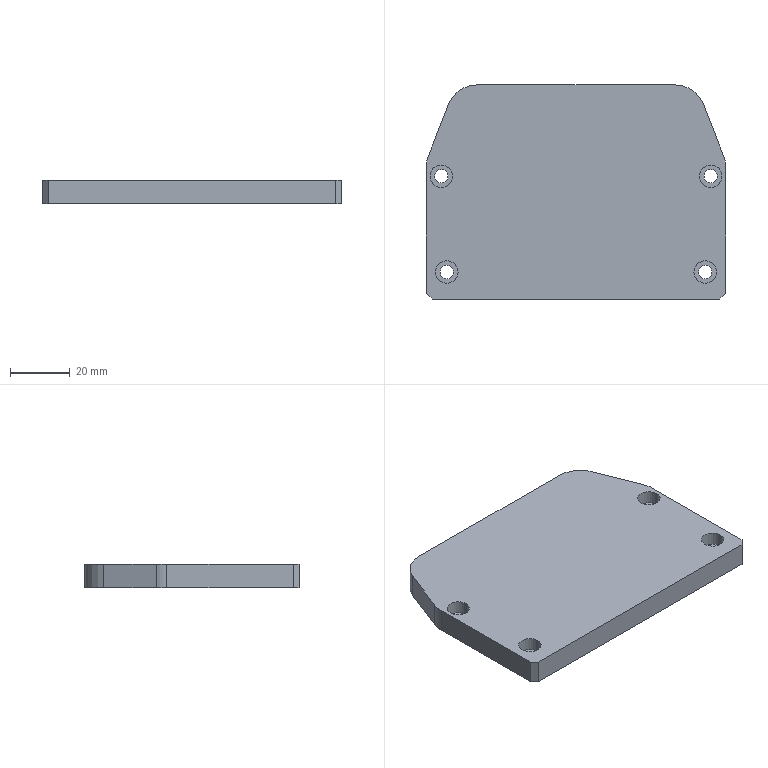Part | SolidWorks | features Chamfer 1, Cut 1, Extrusion 1, Fillet 1, HoleWzd 1, ICE 1 | 1 solid | 37 faces | box 100 x 71.5 x 8 mm | volume 49163 mm3 | cylinder 22 | plane 15 | commonest cylinder face diameters 4.5 x8 7.5 x8 20 x4 35 x2
STEP:
#1=CARTESIAN_POINT('',(-48.75,5.25,3.5));
#2=VERTEX_POINT('',#1);
#3=CARTESIAN_POINT('',(-41.25,5.25,3.5));
#4=VERTEX_POINT('',#3);
#5=CARTESIAN_POINT('',(-45.,5.25,3.5));
#6=DIRECTION('',(0.,0.,1.));
#7=DIRECTION('',(1.,0.,0.));
#8=AXIS2_PLACEMENT_3D('',#5,#6,#7);
#9=CIRCLE('',#8,3.75);
#10=EDGE_CURVE('',#2,#4,#9,.T.);
#11=ORIENTED_EDGE('',*,*,#10,.F.);
#12=CARTESIAN_POINT('',(-48.75,5.25,8.));
#13=VERTEX_POINT('',#12);
#14=CARTESIAN_POINT('',(-48.75,5.25,8.));
#15=DIRECTION('',(0.,0.,1.));
#16=VECTOR('',#15,1000.);
#17=LINE('',#14,#16);
#18=EDGE_CURVE('',#2,#13,#17,.T.);
#19=ORIENTED_EDGE('',*,*,#18,.T.);
#20=CARTESIAN_POINT('',(-41.25,5.25,8.));
#21=VERTEX_POINT('',#20);
#22=CARTESIAN_POINT('',(-45.,5.25,8.));
#23=DIRECTION('',(0.,0.,1.));
#24=DIRECTION('',(1.,0.,0.));
#25=AXIS2_PLACEMENT_3D('',#22,#23,#24);
#26=CIRCLE('',#25,3.75);
#27=EDGE_CURVE('',#13,#21,#26,.T.);
#28=ORIENTED_EDGE('',*,*,#27,.T.);
#29=CARTESIAN_POINT('',(-41.25,5.25,8.));
#30=DIRECTION('',(0.,0.,1.));
#31=VECTOR('',#30,1000.);
#32=LINE('',#29,#31);
#33=EDGE_CURVE('',#4,#21,#32,.T.);
#34=ORIENTED_EDGE('',*,*,#33,.F.);
#35=EDGE_LOOP('',(#11,#19,#28,#34));
#36=FACE_OUTER_BOUND('',#35,.T.);
#37=CARTESIAN_POINT('',(-45.,5.25,8.));
#38=DIRECTION('',(0.,0.,1.));
#39=DIRECTION('',(1.,0.,0.));
#40=AXIS2_PLACEMENT_3D('',#37,#38,#39);
#41=CYLINDRICAL_SURFACE('',#40,3.75);
#42=ADVANCED_FACE('',(#36),#41,.F.);
#43=CARTESIAN_POINT('',(-47.25,5.25,0.));
#44=VERTEX_POINT('',#43);
#45=CARTESIAN_POINT('',(-42.75,5.25,0.));
#46=VERTEX_POINT('',#45);
#47=CARTESIAN_POINT('',(-45.,5.25,0.));
#48=DIRECTION('',(0.,0.,1.));
#49=DIRECTION('',(1.,0.,0.));
#50=AXIS2_PLACEMENT_3D('',#47,#48,#49);
#51=CIRCLE('',#50,2.25);
#52=EDGE_CURVE('',#44,#46,#51,.T.);
#53=ORIENTED_EDGE('',*,*,#52,.F.);
#54=CARTESIAN_POINT('',(-47.25,5.25,3.5));
#55=VERTEX_POINT('',#54);
#56=CARTESIAN_POINT('',(-47.25,5.25,8.));
#57=DIRECTION('',(0.,0.,1.));
#58=VECTOR('',#57,1000.);
#59=LINE('',#56,#58);
#60=EDGE_CURVE('',#44,#55,#59,.T.);
#61=ORIENTED_EDGE('',*,*,#60,.T.);
#62=CARTESIAN_POINT('',(-42.75,5.25,3.5));
#63=VERTEX_POINT('',#62);
#64=CARTESIAN_POINT('',(-45.,5.25,3.5));
#65=DIRECTION('',(0.,0.,1.));
#66=DIRECTION('',(1.,0.,0.));
#67=AXIS2_PLACEMENT_3D('',#64,#65,#66);
#68=CIRCLE('',#67,2.25);
#69=EDGE_CURVE('',#55,#63,#68,.T.);
#70=ORIENTED_EDGE('',*,*,#69,.T.);
#71=CARTESIAN_POINT('',(-42.75,5.25,8.));
#72=DIRECTION('',(0.,0.,1.));
#73=VECTOR('',#72,1000.);
#74=LINE('',#71,#73);
#75=EDGE_CURVE('',#46,#63,#74,.T.);
#76=ORIENTED_EDGE('',*,*,#75,.F.);
#77=EDGE_LOOP('',(#53,#61,#70,#76));
#78=FACE_OUTER_BOUND('',#77,.T.);
#79=CARTESIAN_POINT('',(-45.,5.25,8.));
#80=DIRECTION('',(0.,0.,1.));
#81=DIRECTION('',(1.,0.,0.));
#82=AXIS2_PLACEMENT_3D('',#79,#80,#81);
#83=CYLINDRICAL_SURFACE('',#82,2.25);
#84=ADVANCED_FACE('',(#78),#83,.F.);
#85=CARTESIAN_POINT('',(-46.9,-26.75,3.5));
#86=VERTEX_POINT('',#85);
#87=CARTESIAN_POINT('',(-39.4,-26.75,3.5));
#88=VERTEX_POINT('',#87);
#89=CARTESIAN_POINT('',(-43.15,-26.75,3.5));
#90=DIRECTION('',(0.,0.,1.));
#91=DIRECTION('',(1.,0.,0.));
#92=AXIS2_PLACEMENT_3D('',#89,#90,#91);
#93=CIRCLE('',#92,3.75);
#94=EDGE_CURVE('',#86,#88,#93,.T.);
#95=ORIENTED_EDGE('',*,*,#94,.F.);
#96=CARTESIAN_POINT('',(-46.9,-26.75,8.));
#97=VERTEX_POINT('',#96);
#98=CARTESIAN_POINT('',(-46.9,-26.75,8.));
#99=DIRECTION('',(0.,0.,1.));
#100=VECTOR('',#99,1000.);
#101=LINE('',#98,#100);
#102=EDGE_CURVE('',#86,#97,#101,.T.);
#103=ORIENTED_EDGE('',*,*,#102,.T.);
#104=CARTESIAN_POINT('',(-39.4,-26.75,8.));
#105=VERTEX_POINT('',#104);
#106=CARTESIAN_POINT('',(-43.15,-26.75,8.));
#107=DIRECTION('',(0.,0.,1.));
#108=DIRECTION('',(1.,0.,0.));
#109=AXIS2_PLACEMENT_3D('',#106,#107,#108);
#110=CIRCLE('',#109,3.75);
#111=EDGE_CURVE('',#97,#105,#110,.T.);
#112=ORIENTED_EDGE('',*,*,#111,.T.);
#113=CARTESIAN_POINT('',(-39.4,-26.75,8.));
#114=DIRECTION('',(0.,0.,1.));
#115=VECTOR('',#114,1000.);
#116=LINE('',#113,#115);
#117=EDGE_CURVE('',#88,#105,#116,.T.);
#118=ORIENTED_EDGE('',*,*,#117,.F.);
#119=EDGE_LOOP('',(#95,#103,#112,#118));
#120=FACE_OUTER_BOUND('',#119,.T.);
#121=CARTESIAN_POINT('',(-43.15,-26.75,8.));
#122=DIRECTION('',(0.,0.,1.));
#123=DIRECTION('',(1.,0.,0.));
#124=AXIS2_PLACEMENT_3D('',#121,#122,#123);
#125=CYLINDRICAL_SURFACE('',#124,3.75);
#126=ADVANCED_FACE('',(#120),#125,.F.);
#127=CARTESIAN_POINT('',(-45.4,-26.75,0.));
#128=VERTEX_POINT('',#127);
#129=CARTESIAN_POINT('',(-40.9,-26.75,0.));
#130=VERTEX_POINT('',#129);
#131=CARTESIAN_POINT('',(-43.15,-26.75,0.));
#132=DIRECTION('',(0.,0.,1.));
#133=DIRECTION('',(1.,0.,0.));
#134=AXIS2_PLACEMENT_3D('',#131,#132,#133);
#135=CIRCLE('',#134,2.25);
#136=EDGE_CURVE('',#128,#130,#135,.T.);
#137=ORIENTED_EDGE('',*,*,#136,.F.);
#138=CARTESIAN_POINT('',(-45.4,-26.75,3.5));
#139=VERTEX_POINT('',#138);
#140=CARTESIAN_POINT('',(-45.4,-26.75,8.));
#141=DIRECTION('',(0.,0.,1.));
#142=VECTOR('',#141,1000.);
#143=LINE('',#140,#142);
#144=EDGE_CURVE('',#128,#139,#143,.T.);
#145=ORIENTED_EDGE('',*,*,#144,.T.);
#146=CARTESIAN_POINT('',(-40.9,-26.75,3.5));
#147=VERTEX_POINT('',#146);
#148=CARTESIAN_POINT('',(-43.15,-26.75,3.5));
#149=DIRECTION('',(0.,0.,1.));
#150=DIRECTION('',(1.,0.,0.));
#151=AXIS2_PLACEMENT_3D('',#148,#149,#150);
#152=CIRCLE('',#151,2.25);
#153=EDGE_CURVE('',#139,#147,#152,.T.);
#154=ORIENTED_EDGE('',*,*,#153,.T.);
#155=CARTESIAN_POINT('',(-40.9,-26.75,8.));
#156=DIRECTION('',(0.,0.,1.));
#157=VECTOR('',#156,1000.);
#158=LINE('',#155,#157);
#159=EDGE_CURVE('',#130,#147,#158,.T.);
#160=ORIENTED_EDGE('',*,*,#159,.F.);
#161=EDGE_LOOP('',(#137,#145,#154,#160));
#162=FACE_OUTER_BOUND('',#161,.T.);
#163=CARTESIAN_POINT('',(-43.15,-26.75,8.));
#164=DIRECTION('',(0.,0.,1.));
#165=DIRECTION('',(1.,0.,0.));
#166=AXIS2_PLACEMENT_3D('',#163,#164,#165);
#167=CYLINDRICAL_SURFACE('',#166,2.25);
#168=ADVANCED_FACE('',(#162),#167,.F.);
#169=CARTESIAN_POINT('',(41.25,5.25,3.5));
#170=VERTEX_POINT('',#169);
#171=CARTESIAN_POINT('',(48.75,5.25,3.5));
#172=VERTEX_POINT('',#171);
#173=CARTESIAN_POINT('',(45.,5.25,3.5));
#174=DIRECTION('',(0.,0.,1.));
#175=DIRECTION('',(1.,0.,0.));
#176=AXIS2_PLACEMENT_3D('',#173,#174,#175);
#177=CIRCLE('',#176,3.75);
#178=EDGE_CURVE('',#170,#172,#177,.T.);
#179=ORIENTED_EDGE('',*,*,#178,.F.);
#180=CARTESIAN_POINT('',(41.25,5.25,8.));
#181=VERTEX_POINT('',#180);
#182=CARTESIAN_POINT('',(41.25,5.25,8.));
#183=DIRECTION('',(0.,0.,1.));
#184=VECTOR('',#183,1000.);
#185=LINE('',#182,#184);
#186=EDGE_CURVE('',#170,#181,#185,.T.);
#187=ORIENTED_EDGE('',*,*,#186,.T.);
#188=CARTESIAN_POINT('',(48.75,5.25,8.));
#189=VERTEX_POINT('',#188);
#190=CARTESIAN_POINT('',(45.,5.25,8.));
#191=DIRECTION('',(0.,0.,1.));
#192=DIRECTION('',(1.,0.,0.));
#193=AXIS2_PLACEMENT_3D('',#190,#191,#192);
#194=CIRCLE('',#193,3.75);
#195=EDGE_CURVE('',#181,#189,#194,.T.);
#196=ORIENTED_EDGE('',*,*,#195,.T.);
#197=CARTESIAN_POINT('',(48.75,5.25,8.));
#198=DIRECTION('',(0.,0.,1.));
#199=VECTOR('',#198,1000.);
#200=LINE('',#197,#199);
#201=EDGE_CURVE('',#172,#189,#200,.T.);
#202=ORIENTED_EDGE('',*,*,#201,.F.);
#203=EDGE_LOOP('',(#179,#187,#196,#202));
#204=FACE_OUTER_BOUND('',#203,.T.);
#205=CARTESIAN_POINT('',(45.,5.25,8.));
#206=DIRECTION('',(0.,0.,1.));
#207=DIRECTION('',(1.,0.,0.));
#208=AXIS2_PLACEMENT_3D('',#205,#206,#207);
#209=CYLINDRICAL_SURFACE('',#208,3.75);
#210=ADVANCED_FACE('',(#204),#209,.F.);
#211=CARTESIAN_POINT('',(42.75,5.25,0.));
#212=VERTEX_POINT('',#211);
#213=CARTESIAN_POINT('',(47.25,5.25,0.));
#214=VERTEX_POINT('',#213);
#215=CARTESIAN_POINT('',(45.,5.25,0.));
#216=DIRECTION('',(0.,0.,1.));
#217=DIRECTION('',(1.,0.,0.));
#218=AXIS2_PLACEMENT_3D('',#215,#216,#217);
#219=CIRCLE('',#218,2.25);
#220=EDGE_CURVE('',#212,#214,#219,.T.);
#221=ORIENTED_EDGE('',*,*,#220,.F.);
#222=CARTESIAN_POINT('',(42.75,5.25,3.5));
#223=VERTEX_POINT('',#222);
#224=CARTESIAN_POINT('',(42.75,5.25,8.));
#225=DIRECTION('',(0.,0.,1.));
#226=VECTOR('',#225,1000.);
#227=LINE('',#224,#226);
#228=EDGE_CURVE('',#212,#223,#227,.T.);
#229=ORIENTED_EDGE('',*,*,#228,.T.);
#230=CARTESIAN_POINT('',(47.25,5.25,3.5));
#231=VERTEX_POINT('',#230);
#232=CARTESIAN_POINT('',(45.,5.25,3.5));
#233=DIRECTION('',(0.,0.,1.));
#234=DIRECTION('',(1.,0.,0.));
#235=AXIS2_PLACEMENT_3D('',#232,#233,#234);
#236=CIRCLE('',#235,2.25);
#237=EDGE_CURVE('',#223,#231,#236,.T.);
#238=ORIENTED_EDGE('',*,*,#237,.T.);
#239=CARTESIAN_POINT('',(47.25,5.25,8.));
#240=DIRECTION('',(0.,0.,1.));
#241=VECTOR('',#240,1000.);
#242=LINE('',#239,#241);
#243=EDGE_CURVE('',#214,#231,#242,.T.);
#244=ORIENTED_EDGE('',*,*,#243,.F.);
#245=EDGE_LOOP('',(#221,#229,#238,#244));
#246=FACE_OUTER_BOUND('',#245,.T.);
#247=CARTESIAN_POINT('',(45.,5.25,8.));
#248=DIRECTION('',(0.,0.,1.));
#249=DIRECTION('',(1.,0.,0.));
#250=AXIS2_PLACEMENT_3D('',#247,#248,#249);
#251=CYLINDRICAL_SURFACE('',#250,2.25);
#252=ADVANCED_FACE('',(#246),#251,.F.);
#253=CARTESIAN_POINT('',(39.4,-26.75,3.5));
#254=VERTEX_POINT('',#253);
#255=CARTESIAN_POINT('',(46.9,-26.75,3.5));
#256=VERTEX_POINT('',#255);
#257=CARTESIAN_POINT('',(43.15,-26.75,3.5));
#258=DIRECTION('',(0.,0.,1.));
#259=DIRECTION('',(1.,0.,0.));
#260=AXIS2_PLACEMENT_3D('',#257,#258,#259);
#261=CIRCLE('',#260,3.75);
#262=EDGE_CURVE('',#254,#256,#261,.T.);
#263=ORIENTED_EDGE('',*,*,#262,.F.);
#264=CARTESIAN_POINT('',(39.4,-26.75,8.));
#265=VERTEX_POINT('',#264);
#266=CARTESIAN_POINT('',(39.4,-26.75,8.));
#267=DIRECTION('',(0.,0.,1.));
#268=VECTOR('',#267,1000.);
#269=LINE('',#266,#268);
#270=EDGE_CURVE('',#254,#265,#269,.T.);
#271=ORIENTED_EDGE('',*,*,#270,.T.);
#272=CARTESIAN_POINT('',(46.9,-26.75,8.));
#273=VERTEX_POINT('',#272);
#274=CARTESIAN_POINT('',(43.15,-26.75,8.));
#275=DIRECTION('',(0.,0.,1.));
#276=DIRECTION('',(1.,0.,0.));
#277=AXIS2_PLACEMENT_3D('',#274,#275,#276);
#278=CIRCLE('',#277,3.75);
#279=EDGE_CURVE('',#265,#273,#278,.T.);
#280=ORIENTED_EDGE('',*,*,#279,.T.);
#281=CARTESIAN_POINT('',(46.9,-26.75,8.));
#282=DIRECTION('',(0.,0.,1.));
#283=VECTOR('',#282,1000.);
#284=LINE('',#281,#283);
#285=EDGE_CURVE('',#256,#273,#284,.T.);
#286=ORIENTED_EDGE('',*,*,#285,.F.);
#287=EDGE_LOOP('',(#263,#271,#280,#286));
#288=FACE_OUTER_BOUND('',#287,.T.);
#289=CARTESIAN_POINT('',(43.15,-26.75,8.));
#290=DIRECTION('',(0.,0.,1.));
#291=DIRECTION('',(1.,0.,0.));
#292=AXIS2_PLACEMENT_3D('',#289,#290,#291);
#293=CYLINDRICAL_SURFACE('',#292,3.75);
#294=ADVANCED_FACE('',(#288),#293,.F.);
#295=CARTESIAN_POINT('',(40.9,-26.75,0.));
#296=VERTEX_POINT('',#295);
#297=CARTESIAN_POINT('',(45.4,-26.75,0.));
#298=VERTEX_POINT('',#297);
#299=CARTESIAN_POINT('',(43.15,-26.75,0.));
#300=DIRECTION('',(0.,0.,1.));
#301=DIRECTION('',(1.,0.,0.));
#302=AXIS2_PLACEMENT_3D('',#299,#300,#301);
#303=CIRCLE('',#302,2.25);
#304=EDGE_CURVE('',#296,#298,#303,.T.);
#305=ORIENTED_EDGE('',*,*,#304,.F.);
#306=CARTESIAN_POINT('',(40.9,-26.75,3.5));
#307=VERTEX_POINT('',#306);
#308=CARTESIAN_POINT('',(40.9,-26.75,8.));
#309=DIRECTION('',(0.,0.,1.));
#310=VECTOR('',#309,1000.);
#311=LINE('',#308,#310);
#312=EDGE_CURVE('',#296,#307,#311,.T.);
#313=ORIENTED_EDGE('',*,*,#312,.T.);
#314=CARTESIAN_POINT('',(45.4,-26.75,3.5));
#315=VERTEX_POINT('',#314);
#316=CARTESIAN_POINT('',(43.15,-26.75,3.5));
#317=DIRECTION('',(0.,0.,1.));
#318=DIRECTION('',(1.,0.,0.));
#319=AXIS2_PLACEMENT_3D('',#316,#317,#318);
#320=CIRCLE('',#319,2.25);
#321=EDGE_CURVE('',#307,#315,#320,.T.);
#322=ORIENTED_EDGE('',*,*,#321,.T.);
#323=CARTESIAN_POINT('',(45.4,-26.75,8.));
#324=DIRECTION('',(0.,0.,1.));
#325=VECTOR('',#324,1000.);
#326=LINE('',#323,#325);
#327=EDGE_CURVE('',#298,#315,#326,.T.);
#328=ORIENTED_EDGE('',*,*,#327,.F.);
#329=EDGE_LOOP('',(#305,#313,#322,#328));
#330=FACE_OUTER_BOUND('',#329,.T.);
#331=CARTESIAN_POINT('',(43.15,-26.75,8.));
#332=DIRECTION('',(0.,0.,1.));
#333=DIRECTION('',(1.,0.,0.));
#334=AXIS2_PLACEMENT_3D('',#331,#332,#333);
#335=CYLINDRICAL_SURFACE('',#334,2.25);
#336=ADVANCED_FACE('',(#330),#335,.F.);
#337=CARTESIAN_POINT('',(17.5,8.75,5.));
#338=VERTEX_POINT('',#337);
#339=CARTESIAN_POINT('',(-17.5,8.75,5.));
#340=VERTEX_POINT('',#339);
#341=CARTESIAN_POINT('',(0.,8.75,5.));
#342=DIRECTION('',(0.,0.,-1.));
#343=DIRECTION('',(-1.,0.,0.));
#344=AXIS2_PLACEMENT_3D('',#341,#342,#343);
#345=CIRCLE('',#344,17.5);
#346=EDGE_CURVE('',#338,#340,#345,.T.);
#347=ORIENTED_EDGE('',*,*,#346,.F.);
#348=CARTESIAN_POINT('',(17.5,8.75,0.));
#349=VERTEX_POINT('',#348);
#350=CARTESIAN_POINT('',(17.5,8.75,5.));
#351=DIRECTION('',(0.,0.,-1.));
#352=VECTOR('',#351,1000.);
#353=LINE('',#350,#352);
#354=EDGE_CURVE('',#338,#349,#353,.T.);
#355=ORIENTED_EDGE('',*,*,#354,.T.);
#356=CARTESIAN_POINT('',(-17.5,8.75,0.));
#357=VERTEX_POINT('',#356);
#358=CARTESIAN_POINT('',(0.,8.75,0.));
#359=DIRECTION('',(0.,0.,-1.));
#360=DIRECTION('',(-1.,0.,0.));
#361=AXIS2_PLACEMENT_3D('',#358,#359,#360);
#362=CIRCLE('',#361,17.5);
#363=EDGE_CURVE('',#349,#357,#362,.T.);
#364=ORIENTED_EDGE('',*,*,#363,.T.);
#365=CARTESIAN_POINT('',(-17.5,8.75,5.));
#366=DIRECTION('',(0.,0.,-1.));
#367=VECTOR('',#366,1000.);
#368=LINE('',#365,#367);
#369=EDGE_CURVE('',#340,#357,#368,.T.);
#370=ORIENTED_EDGE('',*,*,#369,.F.);
#371=EDGE_LOOP('',(#347,#355,#364,#370));
#372=FACE_OUTER_BOUND('',#371,.T.);
#373=CARTESIAN_POINT('',(0.,8.75,5.));
#374=DIRECTION('',(0.,0.,-1.));
#375=DIRECTION('',(-1.,0.,0.));
#376=AXIS2_PLACEMENT_3D('',#373,#374,#375);
#377=CYLINDRICAL_SURFACE('',#376,17.5);
#378=ADVANCED_FACE('',(#372),#377,.F.);
#379=CARTESIAN_POINT('',(50.,-33.75,8.));
#380=VERTEX_POINT('',#379);
#381=CARTESIAN_POINT('',(50.,8.359,8.));
#382=VERTEX_POINT('',#381);
#383=CARTESIAN_POINT('',(50.,-35.75,8.));
#384=DIRECTION('',(0.,1.,0.));
#385=VECTOR('',#384,1000.);
#386=LINE('',#383,#385);
#387=EDGE_CURVE('',#380,#382,#386,.T.);
#388=ORIENTED_EDGE('',*,*,#387,.F.);
#389=CARTESIAN_POINT('',(50.,-33.75,0.));
#390=VERTEX_POINT('',#389);
#391=CARTESIAN_POINT('',(50.,-33.75,8.));
#392=DIRECTION('',(0.,0.,-1.));
#393=VECTOR('',#392,1000.);
#394=LINE('',#391,#393);
#395=EDGE_CURVE('',#380,#390,#394,.T.);
#396=ORIENTED_EDGE('',*,*,#395,.T.);
#397=CARTESIAN_POINT('',(50.,8.359,0.));
#398=VERTEX_POINT('',#397);
#399=CARTESIAN_POINT('',(50.,-35.75,0.));
#400=DIRECTION('',(0.,1.,0.));
#401=VECTOR('',#400,1000.);
#402=LINE('',#399,#401);
#403=EDGE_CURVE('',#390,#398,#402,.T.);
#404=ORIENTED_EDGE('',*,*,#403,.T.);
#405=CARTESIAN_POINT('',(50.,8.359,8.));
#406=DIRECTION('',(0.,0.,1.));
#407=VECTOR('',#406,1000.);
#408=LINE('',#405,#407);
#409=EDGE_CURVE('',#398,#382,#408,.T.);
#410=ORIENTED_EDGE('',*,*,#409,.T.);
#411=EDGE_LOOP('',(#388,#396,#404,#410));
#412=FACE_OUTER_BOUND('',#411,.T.);
#413=CARTESIAN_POINT('',(50.,-35.75,8.));
#414=DIRECTION('',(-1.,0.,0.));
#415=DIRECTION('',(0.,0.,1.));
#416=AXIS2_PLACEMENT_3D('',#413,#414,#415);
#417=PLANE('',#416);
#418=ADVANCED_FACE('',(#412),#417,.F.);
#419=CARTESIAN_POINT('',(33.18,35.75,0.));
#420=VERTEX_POINT('',#419);
#421=CARTESIAN_POINT('',(-33.18,35.75,0.));
#422=VERTEX_POINT('',#421);
#423=CARTESIAN_POINT('',(-50.,35.75,0.));
#424=DIRECTION('',(-1.,0.,0.));
#425=VECTOR('',#424,1000.);
#426=LINE('',#423,#425);
#427=EDGE_CURVE('',#420,#422,#426,.T.);
#428=ORIENTED_EDGE('',*,*,#427,.T.);
#429=CARTESIAN_POINT('',(-33.18,35.75,8.));
#430=VERTEX_POINT('',#429);
#431=CARTESIAN_POINT('',(-33.18,35.75,8.));
#432=DIRECTION('',(0.,0.,1.));
#433=VECTOR('',#432,1000.);
#434=LINE('',#431,#433);
#435=EDGE_CURVE('',#422,#430,#434,.T.);
#436=ORIENTED_EDGE('',*,*,#435,.T.);
#437=CARTESIAN_POINT('',(33.18,35.75,8.));
#438=VERTEX_POINT('',#437);
#439=CARTESIAN_POINT('',(-50.,35.75,8.));
#440=DIRECTION('',(-1.,0.,0.));
#441=VECTOR('',#440,1000.);
#442=LINE('',#439,#441);
#443=EDGE_CURVE('',#438,#430,#442,.T.);
#444=ORIENTED_EDGE('',*,*,#443,.F.);
#445=CARTESIAN_POINT('',(33.18,35.75,8.));
#446=DIRECTION('',(0.,0.,-1.));
#447=VECTOR('',#446,1000.);
#448=LINE('',#445,#447);
#449=EDGE_CURVE('',#438,#420,#448,.T.);
#450=ORIENTED_EDGE('',*,*,#449,.T.);
#451=EDGE_LOOP('',(#428,#436,#444,#450));
#452=FACE_OUTER_BOUND('',#451,.T.);
#453=CARTESIAN_POINT('',(-50.,35.75,8.));
#454=DIRECTION('',(0.,-1.,0.));
#455=DIRECTION('',(0.,0.,-1.));
#456=AXIS2_PLACEMENT_3D('',#453,#454,#455);
#457=PLANE('',#456);
#458=ADVANCED_FACE('',(#452),#457,.F.);
#459=CARTESIAN_POINT('',(-50.,8.359,0.));
#460=VERTEX_POINT('',#459);
#461=CARTESIAN_POINT('',(-50.,-33.75,0.));
#462=VERTEX_POINT('',#461);
#463=CARTESIAN_POINT('',(-50.,-35.75,0.));
#464=DIRECTION('',(0.,-1.,0.));
#465=VECTOR('',#464,1000.);
#466=LINE('',#463,#465);
#467=EDGE_CURVE('',#460,#462,#466,.T.);
#468=ORIENTED_EDGE('',*,*,#467,.T.);
#469=CARTESIAN_POINT('',(-50.,-33.75,8.));
#470=VERTEX_POINT('',#469);
#471=CARTESIAN_POINT('',(-50.,-33.75,8.));
#472=DIRECTION('',(0.,0.,1.));
#473=VECTOR('',#472,1000.);
#474=LINE('',#471,#473);
#475=EDGE_CURVE('',#462,#470,#474,.T.);
#476=ORIENTED_EDGE('',*,*,#475,.T.);
#477=CARTESIAN_POINT('',(-50.,8.359,8.));
#478=VERTEX_POINT('',#477);
#479=CARTESIAN_POINT('',(-50.,-35.75,8.));
#480=DIRECTION('',(0.,-1.,0.));
#481=VECTOR('',#480,1000.);
#482=LINE('',#479,#481);
#483=EDGE_CURVE('',#478,#470,#482,.T.);
#484=ORIENTED_EDGE('',*,*,#483,.F.);
#485=CARTESIAN_POINT('',(-50.,8.359,8.));
#486=DIRECTION('',(0.,0.,-1.));
#487=VECTOR('',#486,1000.);
#488=LINE('',#485,#487);
#489=EDGE_CURVE('',#478,#460,#488,.T.);
#490=ORIENTED_EDGE('',*,*,#489,.T.);
#491=EDGE_LOOP('',(#468,#476,#484,#490));
#492=FACE_OUTER_BOUND('',#491,.T.);
#493=CARTESIAN_POINT('',(-50.,-35.75,8.));
#494=DIRECTION('',(1.,0.,0.));
#495=DIRECTION('',(0.,0.,-1.));
#496=AXIS2_PLACEMENT_3D('',#493,#494,#495);
#497=PLANE('',#496);
#498=ADVANCED_FACE('',(#492),#497,.F.);
#499=CARTESIAN_POINT('',(-48.,-35.75,8.));
#500=VERTEX_POINT('',#499);
#501=CARTESIAN_POINT('',(48.,-35.75,8.));
#502=VERTEX_POINT('',#501);
#503=CARTESIAN_POINT('',(-50.,-35.75,8.));
#504=DIRECTION('',(1.,0.,0.));
#505=VECTOR('',#504,1000.);
#506=LINE('',#503,#505);
#507=EDGE_CURVE('',#500,#502,#506,.T.);
#508=ORIENTED_EDGE('',*,*,#507,.F.);
#509=CARTESIAN_POINT('',(-48.,-35.75,0.));
#510=VERTEX_POINT('',#509);
#511=CARTESIAN_POINT('',(-48.,-35.75,8.));
#512=DIRECTION('',(0.,0.,-1.));
#513=VECTOR('',#512,1000.);
#514=LINE('',#511,#513);
#515=EDGE_CURVE('',#500,#510,#514,.T.);
#516=ORIENTED_EDGE('',*,*,#515,.T.);
#517=CARTESIAN_POINT('',(48.,-35.75,0.));
#518=VERTEX_POINT('',#517);
#519=CARTESIAN_POINT('',(-50.,-35.75,0.));
#520=DIRECTION('',(1.,0.,0.));
#521=VECTOR('',#520,1000.);
#522=LINE('',#519,#521);
#523=EDGE_CURVE('',#510,#518,#522,.T.);
#524=ORIENTED_EDGE('',*,*,#523,.T.);
#525=CARTESIAN_POINT('',(48.,-35.75,8.));
#526=DIRECTION('',(0.,0.,1.));
#527=VECTOR('',#526,1000.);
#528=LINE('',#525,#527);
#529=EDGE_CURVE('',#518,#502,#528,.T.);
#530=ORIENTED_EDGE('',*,*,#529,.T.);
#531=EDGE_LOOP('',(#508,#516,#524,#530));
#532=FACE_OUTER_BOUND('',#531,.T.);
#533=CARTESIAN_POINT('',(-50.,-35.75,8.));
#534=DIRECTION('',(0.,1.,0.));
#535=DIRECTION('',(0.,0.,1.));
#536=AXIS2_PLACEMENT_3D('',#533,#534,#535);
#537=PLANE('',#536);
#538=ADVANCED_FACE('',(#532),#537,.F.);
#539=CARTESIAN_POINT('',(-45.,5.25,8.));
#540=DIRECTION('',(0.,0.,1.));
#541=DIRECTION('',(1.,0.,0.));
#542=AXIS2_PLACEMENT_3D('',#539,#540,#541);
#543=CIRCLE('',#542,3.75);
#544=EDGE_CURVE('',#21,#13,#543,.T.);
#545=ORIENTED_EDGE('',*,*,#544,.F.);
#546=ORIENTED_EDGE('',*,*,#27,.F.);
#547=EDGE_LOOP('',(#545,#546));
#548=FACE_BOUND('',#547,.T.);
#549=CARTESIAN_POINT('',(-43.15,-26.75,8.));
#550=DIRECTION('',(0.,0.,1.));
#551=DIRECTION('',(1.,0.,0.));
#552=AXIS2_PLACEMENT_3D('',#549,#550,#551);
#553=CIRCLE('',#552,3.75);
#554=EDGE_CURVE('',#105,#97,#553,.T.);
#555=ORIENTED_EDGE('',*,*,#554,.F.);
#556=ORIENTED_EDGE('',*,*,#111,.F.);
#557=EDGE_LOOP('',(#555,#556));
#558=FACE_BOUND('',#557,.T.);
#559=CARTESIAN_POINT('',(45.,5.25,8.));
#560=DIRECTION('',(0.,0.,1.));
#561=DIRECTION('',(1.,0.,0.));
#562=AXIS2_PLACEMENT_3D('',#559,#560,#561);
#563=CIRCLE('',#562,3.75);
#564=EDGE_CURVE('',#189,#181,#563,.T.);
#565=ORIENTED_EDGE('',*,*,#564,.F.);
#566=ORIENTED_EDGE('',*,*,#195,.F.);
#567=EDGE_LOOP('',(#565,#566));
#568=FACE_BOUND('',#567,.T.);
#569=CARTESIAN_POINT('',(43.15,-26.75,8.));
#570=DIRECTION('',(0.,0.,1.));
#571=DIRECTION('',(1.,0.,0.));
#572=AXIS2_PLACEMENT_3D('',#569,#570,#571);
#573=CIRCLE('',#572,3.75);
#574=EDGE_CURVE('',#273,#265,#573,.T.);
#575=ORIENTED_EDGE('',*,*,#574,.F.);
#576=ORIENTED_EDGE('',*,*,#279,.F.);
#577=EDGE_LOOP('',(#575,#576));
#578=FACE_BOUND('',#577,.T.);
#579=ORIENTED_EDGE('',*,*,#483,.T.);
#580=CARTESIAN_POINT('',(-48.,-35.75,8.));
#581=DIRECTION('',(0.7071,-0.7071,0.));
#582=VECTOR('',#581,1000.);
#583=LINE('',#580,#582);
#584=EDGE_CURVE('',#470,#500,#583,.T.);
#585=ORIENTED_EDGE('',*,*,#584,.T.);
#586=ORIENTED_EDGE('',*,*,#507,.T.);
#587=CARTESIAN_POINT('',(50.,-33.75,8.));
#588=DIRECTION('',(0.7071,0.7071,0.));
#589=VECTOR('',#588,1000.);
#590=LINE('',#587,#589);
#591=EDGE_CURVE('',#502,#380,#590,.T.);
#592=ORIENTED_EDGE('',*,*,#591,.T.);
#593=ORIENTED_EDGE('',*,*,#387,.T.);
#594=CARTESIAN_POINT('',(49.31,12.01,8.));
#595=VERTEX_POINT('',#594);
#596=CARTESIAN_POINT('',(40.,8.359,8.));
#597=DIRECTION('',(0.,0.,1.));
#598=DIRECTION('',(-1.,0.,0.));
#599=AXIS2_PLACEMENT_3D('',#596,#597,#598);
#600=CIRCLE('',#599,10.);
#601=EDGE_CURVE('',#382,#595,#600,.T.);
#602=ORIENTED_EDGE('',*,*,#601,.T.);
#603=CARTESIAN_POINT('',(42.49,29.401,8.));
#604=VERTEX_POINT('',#603);
#605=CARTESIAN_POINT('',(46.819,18.361,8.));
#606=DIRECTION('',(-0.3651,0.931,0.));
#607=VECTOR('',#606,1000.);
#608=LINE('',#605,#607);
#609=EDGE_CURVE('',#595,#604,#608,.T.);
#610=ORIENTED_EDGE('',*,*,#609,.T.);
#611=CARTESIAN_POINT('',(33.18,25.75,8.));
#612=DIRECTION('',(0.,0.,1.));
#613=DIRECTION('',(-1.,0.,0.));
#614=AXIS2_PLACEMENT_3D('',#611,#612,#613);
#615=CIRCLE('',#614,10.);
#616=EDGE_CURVE('',#604,#438,#615,.T.);
#617=ORIENTED_EDGE('',*,*,#616,.T.);
#618=ORIENTED_EDGE('',*,*,#443,.T.);
#619=CARTESIAN_POINT('',(-42.49,29.401,8.));
#620=VERTEX_POINT('',#619);
#621=CARTESIAN_POINT('',(-33.18,25.75,8.));
#622=DIRECTION('',(0.,0.,1.));
#623=DIRECTION('',(-1.,0.,0.));
#624=AXIS2_PLACEMENT_3D('',#621,#622,#623);
#625=CIRCLE('',#624,10.);
#626=EDGE_CURVE('',#430,#620,#625,.T.);
#627=ORIENTED_EDGE('',*,*,#626,.T.);
#628=CARTESIAN_POINT('',(-49.31,12.01,8.));
#629=VERTEX_POINT('',#628);
#630=CARTESIAN_POINT('',(-46.819,18.361,8.));
#631=DIRECTION('',(-0.3651,-0.931,0.));
#632=VECTOR('',#631,1000.);
#633=LINE('',#630,#632);
#634=EDGE_CURVE('',#620,#629,#633,.T.);
#635=ORIENTED_EDGE('',*,*,#634,.T.);
#636=CARTESIAN_POINT('',(-40.,8.359,8.));
#637=DIRECTION('',(0.,0.,1.));
#638=DIRECTION('',(-1.,0.,0.));
#639=AXIS2_PLACEMENT_3D('',#636,#637,#638);
#640=CIRCLE('',#639,10.);
#641=EDGE_CURVE('',#629,#478,#640,.T.);
#642=ORIENTED_EDGE('',*,*,#641,.T.);
#643=EDGE_LOOP('',(#579,#585,#586,#592,#593,#602,#610,#617,#618,#627,#635,#642));
#644=FACE_OUTER_BOUND('',#643,.T.);
#645=CARTESIAN_POINT('',(0.,0.,8.));
#646=DIRECTION('',(0.,0.,-1.));
#647=DIRECTION('',(-1.,0.,0.));
#648=AXIS2_PLACEMENT_3D('',#645,#646,#647);
#649=PLANE('',#648);
#650=ADVANCED_FACE('',(#548,#558,#568,#578,#644),#649,.F.);
#651=CARTESIAN_POINT('',(-45.,5.25,0.));
#652=DIRECTION('',(0.,0.,1.));
#653=DIRECTION('',(1.,0.,0.));
#654=AXIS2_PLACEMENT_3D('',#651,#652,#653);
#655=CIRCLE('',#654,2.25);
#656=EDGE_CURVE('',#46,#44,#655,.T.);
#657=ORIENTED_EDGE('',*,*,#656,.T.);
#658=ORIENTED_EDGE('',*,*,#52,.T.);
#659=EDGE_LOOP('',(#657,#658));
#660=FACE_BOUND('',#659,.T.);
#661=CARTESIAN_POINT('',(-43.15,-26.75,0.));
#662=DIRECTION('',(0.,0.,1.));
#663=DIRECTION('',(1.,0.,0.));
#664=AXIS2_PLACEMENT_3D('',#661,#662,#663);
#665=CIRCLE('',#664,2.25);
#666=EDGE_CURVE('',#130,#128,#665,.T.);
#667=ORIENTED_EDGE('',*,*,#666,.T.);
#668=ORIENTED_EDGE('',*,*,#136,.T.);
#669=EDGE_LOOP('',(#667,#668));
#670=FACE_BOUND('',#669,.T.);
#671=CARTESIAN_POINT('',(45.,5.25,0.));
#672=DIRECTION('',(0.,0.,1.));
#673=DIRECTION('',(1.,0.,0.));
#674=AXIS2_PLACEMENT_3D('',#671,#672,#673);
#675=CIRCLE('',#674,2.25);
#676=EDGE_CURVE('',#214,#212,#675,.T.);
#677=ORIENTED_EDGE('',*,*,#676,.T.);
#678=ORIENTED_EDGE('',*,*,#220,.T.);
#679=EDGE_LOOP('',(#677,#678));
#680=FACE_BOUND('',#679,.T.);
#681=CARTESIAN_POINT('',(43.15,-26.75,0.));
#682=DIRECTION('',(0.,0.,1.));
#683=DIRECTION('',(1.,0.,0.));
#684=AXIS2_PLACEMENT_3D('',#681,#682,#683);
#685=CIRCLE('',#684,2.25);
#686=EDGE_CURVE('',#298,#296,#685,.T.);
#687=ORIENTED_EDGE('',*,*,#686,.T.);
#688=ORIENTED_EDGE('',*,*,#304,.T.);
#689=EDGE_LOOP('',(#687,#688));
#690=FACE_BOUND('',#689,.T.);
#691=CARTESIAN_POINT('',(0.,8.75,0.));
#692=DIRECTION('',(0.,0.,-1.));
#693=DIRECTION('',(-1.,0.,0.));
#694=AXIS2_PLACEMENT_3D('',#691,#692,#693);
#695=CIRCLE('',#694,17.5);
#696=EDGE_CURVE('',#357,#349,#695,.T.);
#697=ORIENTED_EDGE('',*,*,#696,.F.);
#698=ORIENTED_EDGE('',*,*,#363,.F.);
#699=EDGE_LOOP('',(#697,#698));
#700=FACE_BOUND('',#699,.T.);
#701=ORIENTED_EDGE('',*,*,#523,.F.);
#702=CARTESIAN_POINT('',(-41.875,-41.875,0.));
#703=DIRECTION('',(-0.7071,0.7071,0.));
#704=VECTOR('',#703,1000.);
#705=LINE('',#702,#704);
#706=EDGE_CURVE('',#510,#462,#705,.T.);
#707=ORIENTED_EDGE('',*,*,#706,.T.);
#708=ORIENTED_EDGE('',*,*,#467,.F.);
#709=CARTESIAN_POINT('',(-49.31,12.01,0.));
#710=VERTEX_POINT('',#709);
#711=CARTESIAN_POINT('',(-40.,8.359,0.));
#712=DIRECTION('',(0.,0.,-1.));
#713=DIRECTION('',(-1.,0.,0.));
#714=AXIS2_PLACEMENT_3D('',#711,#712,#713);
#715=CIRCLE('',#714,10.);
#716=EDGE_CURVE('',#460,#710,#715,.T.);
#717=ORIENTED_EDGE('',*,*,#716,.T.);
#718=CARTESIAN_POINT('',(-42.49,29.401,0.));
#719=VERTEX_POINT('',#718);
#720=CARTESIAN_POINT('',(-50.,10.25,0.));
#721=DIRECTION('',(-0.3651,-0.931,0.));
#722=VECTOR('',#721,1000.);
#723=LINE('',#720,#722);
#724=EDGE_CURVE('',#719,#710,#723,.T.);
#725=ORIENTED_EDGE('',*,*,#724,.F.);
#726=CARTESIAN_POINT('',(-33.18,25.75,0.));
#727=DIRECTION('',(0.,0.,-1.));
#728=DIRECTION('',(-1.,0.,0.));
#729=AXIS2_PLACEMENT_3D('',#726,#727,#728);
#730=CIRCLE('',#729,10.);
#731=EDGE_CURVE('',#719,#422,#730,.T.);
#732=ORIENTED_EDGE('',*,*,#731,.T.);
#733=ORIENTED_EDGE('',*,*,#427,.F.);
#734=CARTESIAN_POINT('',(42.49,29.401,0.));
#735=VERTEX_POINT('',#734);
#736=CARTESIAN_POINT('',(33.18,25.75,0.));
#737=DIRECTION('',(0.,0.,-1.));
#738=DIRECTION('',(-1.,0.,0.));
#739=AXIS2_PLACEMENT_3D('',#736,#737,#738);
#740=CIRCLE('',#739,10.);
#741=EDGE_CURVE('',#420,#735,#740,.T.);
#742=ORIENTED_EDGE('',*,*,#741,.T.);
#743=CARTESIAN_POINT('',(49.31,12.01,0.));
#744=VERTEX_POINT('',#743);
#745=CARTESIAN_POINT('',(50.,10.25,0.));
#746=DIRECTION('',(-0.3651,0.931,0.));
#747=VECTOR('',#746,1000.);
#748=LINE('',#745,#747);
#749=EDGE_CURVE('',#744,#735,#748,.T.);
#750=ORIENTED_EDGE('',*,*,#749,.F.);
#751=CARTESIAN_POINT('',(40.,8.359,0.));
#752=DIRECTION('',(0.,0.,-1.));
#753=DIRECTION('',(-1.,0.,0.));
#754=AXIS2_PLACEMENT_3D('',#751,#752,#753);
#755=CIRCLE('',#754,10.);
#756=EDGE_CURVE('',#744,#398,#755,.T.);
#757=ORIENTED_EDGE('',*,*,#756,.T.);
#758=ORIENTED_EDGE('',*,*,#403,.F.);
#759=CARTESIAN_POINT('',(41.875,-41.875,0.));
#760=DIRECTION('',(-0.7071,-0.7071,0.));
#761=VECTOR('',#760,1000.);
#762=LINE('',#759,#761);
#763=EDGE_CURVE('',#390,#518,#762,.T.);
#764=ORIENTED_EDGE('',*,*,#763,.T.);
#765=EDGE_LOOP('',(#701,#707,#708,#717,#725,#732,#733,#742,#750,#757,#758,#764));
#766=FACE_OUTER_BOUND('',#765,.T.);
#767=CARTESIAN_POINT('',(0.,0.,0.));
#768=DIRECTION('',(0.,0.,-1.));
#769=DIRECTION('',(-1.,0.,0.));
#770=AXIS2_PLACEMENT_3D('',#767,#768,#769);
#771=PLANE('',#770);
#772=ADVANCED_FACE('',(#660,#670,#680,#690,#700,#766),#771,.T.);
#773=ORIENTED_EDGE('',*,*,#749,.T.);
#774=CARTESIAN_POINT('',(42.49,29.401,10.));
#775=DIRECTION('',(0.,0.,1.));
#776=VECTOR('',#775,1000.);
#777=LINE('',#774,#776);
#778=EDGE_CURVE('',#735,#604,#777,.T.);
#779=ORIENTED_EDGE('',*,*,#778,.T.);
#780=ORIENTED_EDGE('',*,*,#609,.F.);
#781=CARTESIAN_POINT('',(49.31,12.01,10.));
#782=DIRECTION('',(0.,0.,-1.));
#783=VECTOR('',#782,1000.);
#784=LINE('',#781,#783);
#785=EDGE_CURVE('',#595,#744,#784,.T.);
#786=ORIENTED_EDGE('',*,*,#785,.T.);
#787=EDGE_LOOP('',(#773,#779,#780,#786));
#788=FACE_OUTER_BOUND('',#787,.T.);
#789=CARTESIAN_POINT('',(50.,10.25,10.));
#790=DIRECTION('',(-0.931,-0.3651,0.));
#791=DIRECTION('',(0.3651,-0.931,0.));
#792=AXIS2_PLACEMENT_3D('',#789,#790,#791);
#793=PLANE('',#792);
#794=ADVANCED_FACE('',(#788),#793,.F.);
#795=ORIENTED_EDGE('',*,*,#724,.T.);
#796=CARTESIAN_POINT('',(-49.31,12.01,10.));
#797=DIRECTION('',(0.,0.,1.));
#798=VECTOR('',#797,1000.);
#799=LINE('',#796,#798);
#800=EDGE_CURVE('',#710,#629,#799,.T.);
#801=ORIENTED_EDGE('',*,*,#800,.T.);
#802=ORIENTED_EDGE('',*,*,#634,.F.);
#803=CARTESIAN_POINT('',(-42.49,29.401,10.));
#804=DIRECTION('',(0.,0.,-1.));
#805=VECTOR('',#804,1000.);
#806=LINE('',#803,#805);
#807=EDGE_CURVE('',#620,#719,#806,.T.);
#808=ORIENTED_EDGE('',*,*,#807,.T.);
#809=EDGE_LOOP('',(#795,#801,#802,#808));
#810=FACE_OUTER_BOUND('',#809,.T.);
#811=CARTESIAN_POINT('',(-50.,10.25,10.));
#812=DIRECTION('',(0.931,-0.3651,0.));
#813=DIRECTION('',(0.3651,0.931,0.));
#814=AXIS2_PLACEMENT_3D('',#811,#812,#813);
#815=PLANE('',#814);
#816=ADVANCED_FACE('',(#810),#815,.F.);
#817=ORIENTED_EDGE('',*,*,#641,.F.);
#818=ORIENTED_EDGE('',*,*,#800,.F.);
#819=ORIENTED_EDGE('',*,*,#716,.F.);
#820=ORIENTED_EDGE('',*,*,#489,.F.);
#821=EDGE_LOOP('',(#817,#818,#819,#820));
#822=FACE_OUTER_BOUND('',#821,.T.);
#823=CARTESIAN_POINT('',(-40.,8.359,8.));
#824=DIRECTION('',(0.,0.,-1.));
#825=DIRECTION('',(-1.,0.,0.));
#826=AXIS2_PLACEMENT_3D('',#823,#824,#825);
#827=CYLINDRICAL_SURFACE('',#826,10.);
#828=ADVANCED_FACE('',(#822),#827,.T.);
#829=ORIENTED_EDGE('',*,*,#626,.F.);
#830=ORIENTED_EDGE('',*,*,#435,.F.);
#831=ORIENTED_EDGE('',*,*,#731,.F.);
#832=ORIENTED_EDGE('',*,*,#807,.F.);
#833=EDGE_LOOP('',(#829,#830,#831,#832));
#834=FACE_OUTER_BOUND('',#833,.T.);
#835=CARTESIAN_POINT('',(-33.18,25.75,10.));
#836=DIRECTION('',(0.,0.,-1.));
#837=DIRECTION('',(-1.,0.,0.));
#838=AXIS2_PLACEMENT_3D('',#835,#836,#837);
#839=CYLINDRICAL_SURFACE('',#838,10.);
#840=ADVANCED_FACE('',(#834),#839,.T.);
#841=ORIENTED_EDGE('',*,*,#616,.F.);
#842=ORIENTED_EDGE('',*,*,#778,.F.);
#843=ORIENTED_EDGE('',*,*,#741,.F.);
#844=ORIENTED_EDGE('',*,*,#449,.F.);
#845=EDGE_LOOP('',(#841,#842,#843,#844));
#846=FACE_OUTER_BOUND('',#845,.T.);
#847=CARTESIAN_POINT('',(33.18,25.75,8.));
#848=DIRECTION('',(0.,0.,-1.));
#849=DIRECTION('',(-1.,0.,0.));
#850=AXIS2_PLACEMENT_3D('',#847,#848,#849);
#851=CYLINDRICAL_SURFACE('',#850,10.);
#852=ADVANCED_FACE('',(#846),#851,.T.);
#853=ORIENTED_EDGE('',*,*,#601,.F.);
#854=ORIENTED_EDGE('',*,*,#409,.F.);
#855=ORIENTED_EDGE('',*,*,#756,.F.);
#856=ORIENTED_EDGE('',*,*,#785,.F.);
#857=EDGE_LOOP('',(#853,#854,#855,#856));
#858=FACE_OUTER_BOUND('',#857,.T.);
#859=CARTESIAN_POINT('',(40.,8.359,10.));
#860=DIRECTION('',(0.,0.,-1.));
#861=DIRECTION('',(-1.,0.,0.));
#862=AXIS2_PLACEMENT_3D('',#859,#860,#861);
#863=CYLINDRICAL_SURFACE('',#862,10.);
#864=ADVANCED_FACE('',(#858),#863,.T.);
#865=ORIENTED_EDGE('',*,*,#584,.F.);
#866=ORIENTED_EDGE('',*,*,#475,.F.);
#867=ORIENTED_EDGE('',*,*,#706,.F.);
#868=ORIENTED_EDGE('',*,*,#515,.F.);
#869=EDGE_LOOP('',(#865,#866,#867,#868));
#870=FACE_OUTER_BOUND('',#869,.T.);
#871=CARTESIAN_POINT('',(-48.,-35.75,8.));
#872=DIRECTION('',(0.7071,0.7071,0.));
#873=DIRECTION('',(0.,0.,-1.));
#874=AXIS2_PLACEMENT_3D('',#871,#872,#873);
#875=PLANE('',#874);
#876=ADVANCED_FACE('',(#870),#875,.F.);
#877=ORIENTED_EDGE('',*,*,#591,.F.);
#878=ORIENTED_EDGE('',*,*,#529,.F.);
#879=ORIENTED_EDGE('',*,*,#763,.F.);
#880=ORIENTED_EDGE('',*,*,#395,.F.);
#881=EDGE_LOOP('',(#877,#878,#879,#880));
#882=FACE_OUTER_BOUND('',#881,.T.);
#883=CARTESIAN_POINT('',(50.,-33.75,8.));
#884=DIRECTION('',(-0.7071,0.7071,0.));
#885=DIRECTION('',(0.,0.,-1.));
#886=AXIS2_PLACEMENT_3D('',#883,#884,#885);
#887=PLANE('',#886);
#888=ADVANCED_FACE('',(#882),#887,.F.);
#889=ORIENTED_EDGE('',*,*,#354,.F.);
#890=CARTESIAN_POINT('',(0.,8.75,5.));
#891=DIRECTION('',(0.,0.,-1.));
#892=DIRECTION('',(-1.,0.,0.));
#893=AXIS2_PLACEMENT_3D('',#890,#891,#892);
#894=CIRCLE('',#893,17.5);
#895=EDGE_CURVE('',#340,#338,#894,.T.);
#896=ORIENTED_EDGE('',*,*,#895,.F.);
#897=ORIENTED_EDGE('',*,*,#369,.T.);
#898=ORIENTED_EDGE('',*,*,#696,.T.);
#899=EDGE_LOOP('',(#889,#896,#897,#898));
#900=FACE_OUTER_BOUND('',#899,.T.);
#901=CARTESIAN_POINT('',(0.,8.75,5.));
#902=DIRECTION('',(0.,0.,-1.));
#903=DIRECTION('',(-1.,0.,0.));
#904=AXIS2_PLACEMENT_3D('',#901,#902,#903);
#905=CYLINDRICAL_SURFACE('',#904,17.5);
#906=ADVANCED_FACE('',(#900),#905,.F.);
#907=ORIENTED_EDGE('',*,*,#895,.T.);
#908=ORIENTED_EDGE('',*,*,#346,.T.);
#909=EDGE_LOOP('',(#907,#908));
#910=FACE_OUTER_BOUND('',#909,.T.);
#911=CARTESIAN_POINT('',(0.,8.75,5.));
#912=DIRECTION('',(0.,0.,-1.));
#913=DIRECTION('',(-1.,0.,0.));
#914=AXIS2_PLACEMENT_3D('',#911,#912,#913);
#915=PLANE('',#914);
#916=ADVANCED_FACE('',(#910),#915,.T.);
#917=ORIENTED_EDGE('',*,*,#312,.F.);
#918=ORIENTED_EDGE('',*,*,#686,.F.);
#919=ORIENTED_EDGE('',*,*,#327,.T.);
#920=CARTESIAN_POINT('',(43.15,-26.75,3.5));
#921=DIRECTION('',(0.,0.,1.));
#922=DIRECTION('',(1.,0.,0.));
#923=AXIS2_PLACEMENT_3D('',#920,#921,#922);
#924=CIRCLE('',#923,2.25);
#925=EDGE_CURVE('',#315,#307,#924,.T.);
#926=ORIENTED_EDGE('',*,*,#925,.T.);
#927=EDGE_LOOP('',(#917,#918,#919,#926));
#928=FACE_OUTER_BOUND('',#927,.T.);
#929=CARTESIAN_POINT('',(43.15,-26.75,8.));
#930=DIRECTION('',(0.,0.,1.));
#931=DIRECTION('',(1.,0.,0.));
#932=AXIS2_PLACEMENT_3D('',#929,#930,#931);
#933=CYLINDRICAL_SURFACE('',#932,2.25);
#934=ADVANCED_FACE('',(#928),#933,.F.);
#935=ORIENTED_EDGE('',*,*,#925,.F.);
#936=ORIENTED_EDGE('',*,*,#321,.F.);
#937=EDGE_LOOP('',(#935,#936));
#938=FACE_BOUND('',#937,.T.);
#939=CARTESIAN_POINT('',(43.15,-26.75,3.5));
#940=DIRECTION('',(0.,0.,1.));
#941=DIRECTION('',(1.,0.,0.));
#942=AXIS2_PLACEMENT_3D('',#939,#940,#941);
#943=CIRCLE('',#942,3.75);
#944=EDGE_CURVE('',#256,#254,#943,.T.);
#945=ORIENTED_EDGE('',*,*,#944,.T.);
#946=ORIENTED_EDGE('',*,*,#262,.T.);
#947=EDGE_LOOP('',(#945,#946));
#948=FACE_OUTER_BOUND('',#947,.T.);
#949=CARTESIAN_POINT('',(45.4,-26.75,3.5));
#950=DIRECTION('',(0.,0.,-1.));
#951=DIRECTION('',(-1.,0.,0.));
#952=AXIS2_PLACEMENT_3D('',#949,#950,#951);
#953=PLANE('',#952);
#954=ADVANCED_FACE('',(#938,#948),#953,.F.);
#955=ORIENTED_EDGE('',*,*,#270,.F.);
#956=ORIENTED_EDGE('',*,*,#944,.F.);
#957=ORIENTED_EDGE('',*,*,#285,.T.);
#958=ORIENTED_EDGE('',*,*,#574,.T.);
#959=EDGE_LOOP('',(#955,#956,#957,#958));
#960=FACE_OUTER_BOUND('',#959,.T.);
#961=CARTESIAN_POINT('',(43.15,-26.75,8.));
#962=DIRECTION('',(0.,0.,1.));
#963=DIRECTION('',(1.,0.,0.));
#964=AXIS2_PLACEMENT_3D('',#961,#962,#963);
#965=CYLINDRICAL_SURFACE('',#964,3.75);
#966=ADVANCED_FACE('',(#960),#965,.F.);
#967=ORIENTED_EDGE('',*,*,#228,.F.);
#968=ORIENTED_EDGE('',*,*,#676,.F.);
#969=ORIENTED_EDGE('',*,*,#243,.T.);
#970=CARTESIAN_POINT('',(45.,5.25,3.5));
#971=DIRECTION('',(0.,0.,1.));
#972=DIRECTION('',(1.,0.,0.));
#973=AXIS2_PLACEMENT_3D('',#970,#971,#972);
#974=CIRCLE('',#973,2.25);
#975=EDGE_CURVE('',#231,#223,#974,.T.);
#976=ORIENTED_EDGE('',*,*,#975,.T.);
#977=EDGE_LOOP('',(#967,#968,#969,#976));
#978=FACE_OUTER_BOUND('',#977,.T.);
#979=CARTESIAN_POINT('',(45.,5.25,8.));
#980=DIRECTION('',(0.,0.,1.));
#981=DIRECTION('',(1.,0.,0.));
#982=AXIS2_PLACEMENT_3D('',#979,#980,#981);
#983=CYLINDRICAL_SURFACE('',#982,2.25);
#984=ADVANCED_FACE('',(#978),#983,.F.);
#985=ORIENTED_EDGE('',*,*,#975,.F.);
#986=ORIENTED_EDGE('',*,*,#237,.F.);
#987=EDGE_LOOP('',(#985,#986));
#988=FACE_BOUND('',#987,.T.);
#989=CARTESIAN_POINT('',(45.,5.25,3.5));
#990=DIRECTION('',(0.,0.,1.));
#991=DIRECTION('',(1.,0.,0.));
#992=AXIS2_PLACEMENT_3D('',#989,#990,#991);
#993=CIRCLE('',#992,3.75);
#994=EDGE_CURVE('',#172,#170,#993,.T.);
#995=ORIENTED_EDGE('',*,*,#994,.T.);
#996=ORIENTED_EDGE('',*,*,#178,.T.);
#997=EDGE_LOOP('',(#995,#996));
#998=FACE_OUTER_BOUND('',#997,.T.);
#999=CARTESIAN_POINT('',(47.25,5.25,3.5));
#1000=DIRECTION('',(0.,0.,-1.));
#1001=DIRECTION('',(-1.,0.,0.));
#1002=AXIS2_PLACEMENT_3D('',#999,#1000,#1001);
#1003=PLANE('',#1002);
#1004=ADVANCED_FACE('',(#988,#998),#1003,.F.);
#1005=ORIENTED_EDGE('',*,*,#186,.F.);
#1006=ORIENTED_EDGE('',*,*,#994,.F.);
#1007=ORIENTED_EDGE('',*,*,#201,.T.);
#1008=ORIENTED_EDGE('',*,*,#564,.T.);
#1009=EDGE_LOOP('',(#1005,#1006,#1007,#1008));
#1010=FACE_OUTER_BOUND('',#1009,.T.);
#1011=CARTESIAN_POINT('',(45.,5.25,8.));
#1012=DIRECTION('',(0.,0.,1.));
#1013=DIRECTION('',(1.,0.,0.));
#1014=AXIS2_PLACEMENT_3D('',#1011,#1012,#1013);
#1015=CYLINDRICAL_SURFACE('',#1014,3.75);
#1016=ADVANCED_FACE('',(#1010),#1015,.F.);
#1017=ORIENTED_EDGE('',*,*,#144,.F.);
#1018=ORIENTED_EDGE('',*,*,#666,.F.);
#1019=ORIENTED_EDGE('',*,*,#159,.T.);
#1020=CARTESIAN_POINT('',(-43.15,-26.75,3.5));
#1021=DIRECTION('',(0.,0.,1.));
#1022=DIRECTION('',(1.,0.,0.));
#1023=AXIS2_PLACEMENT_3D('',#1020,#1021,#1022);
#1024=CIRCLE('',#1023,2.25);
#1025=EDGE_CURVE('',#147,#139,#1024,.T.);
#1026=ORIENTED_EDGE('',*,*,#1025,.T.);
#1027=EDGE_LOOP('',(#1017,#1018,#1019,#1026));
#1028=FACE_OUTER_BOUND('',#1027,.T.);
#1029=CARTESIAN_POINT('',(-43.15,-26.75,8.));
#1030=DIRECTION('',(0.,0.,1.));
#1031=DIRECTION('',(1.,0.,0.));
#1032=AXIS2_PLACEMENT_3D('',#1029,#1030,#1031);
#1033=CYLINDRICAL_SURFACE('',#1032,2.25);
#1034=ADVANCED_FACE('',(#1028),#1033,.F.);
#1035=ORIENTED_EDGE('',*,*,#1025,.F.);
#1036=ORIENTED_EDGE('',*,*,#153,.F.);
#1037=EDGE_LOOP('',(#1035,#1036));
#1038=FACE_BOUND('',#1037,.T.);
#1039=CARTESIAN_POINT('',(-43.15,-26.75,3.5));
#1040=DIRECTION('',(0.,0.,1.));
#1041=DIRECTION('',(1.,0.,0.));
#1042=AXIS2_PLACEMENT_3D('',#1039,#1040,#1041);
#1043=CIRCLE('',#1042,3.75);
#1044=EDGE_CURVE('',#88,#86,#1043,.T.);
#1045=ORIENTED_EDGE('',*,*,#1044,.T.);
#1046=ORIENTED_EDGE('',*,*,#94,.T.);
#1047=EDGE_LOOP('',(#1045,#1046));
#1048=FACE_OUTER_BOUND('',#1047,.T.);
#1049=CARTESIAN_POINT('',(-40.9,-26.75,3.5));
#1050=DIRECTION('',(0.,0.,-1.));
#1051=DIRECTION('',(-1.,0.,0.));
#1052=AXIS2_PLACEMENT_3D('',#1049,#1050,#1051);
#1053=PLANE('',#1052);
#1054=ADVANCED_FACE('',(#1038,#1048),#1053,.F.);
#1055=ORIENTED_EDGE('',*,*,#102,.F.);
#1056=ORIENTED_EDGE('',*,*,#1044,.F.);
#1057=ORIENTED_EDGE('',*,*,#117,.T.);
#1058=ORIENTED_EDGE('',*,*,#554,.T.);
#1059=EDGE_LOOP('',(#1055,#1056,#1057,#1058));
#1060=FACE_OUTER_BOUND('',#1059,.T.);
#1061=CARTESIAN_POINT('',(-43.15,-26.75,8.));
#1062=DIRECTION('',(0.,0.,1.));
#1063=DIRECTION('',(1.,0.,0.));
#1064=AXIS2_PLACEMENT_3D('',#1061,#1062,#1063);
#1065=CYLINDRICAL_SURFACE('',#1064,3.75);
#1066=ADVANCED_FACE('',(#1060),#1065,.F.);
#1067=ORIENTED_EDGE('',*,*,#60,.F.);
#1068=ORIENTED_EDGE('',*,*,#656,.F.);
#1069=ORIENTED_EDGE('',*,*,#75,.T.);
#1070=CARTESIAN_POINT('',(-45.,5.25,3.5));
#1071=DIRECTION('',(0.,0.,1.));
#1072=DIRECTION('',(1.,0.,0.));
#1073=AXIS2_PLACEMENT_3D('',#1070,#1071,#1072);
#1074=CIRCLE('',#1073,2.25);
#1075=EDGE_CURVE('',#63,#55,#1074,.T.);
#1076=ORIENTED_EDGE('',*,*,#1075,.T.);
#1077=EDGE_LOOP('',(#1067,#1068,#1069,#1076));
#1078=FACE_OUTER_BOUND('',#1077,.T.);
#1079=CARTESIAN_POINT('',(-45.,5.25,8.));
#1080=DIRECTION('',(0.,0.,1.));
#1081=DIRECTION('',(1.,0.,0.));
#1082=AXIS2_PLACEMENT_3D('',#1079,#1080,#1081);
#1083=CYLINDRICAL_SURFACE('',#1082,2.25);
#1084=ADVANCED_FACE('',(#1078),#1083,.F.);
#1085=ORIENTED_EDGE('',*,*,#1075,.F.);
#1086=ORIENTED_EDGE('',*,*,#69,.F.);
#1087=EDGE_LOOP('',(#1085,#1086));
#1088=FACE_BOUND('',#1087,.T.);
#1089=CARTESIAN_POINT('',(-45.,5.25,3.5));
#1090=DIRECTION('',(0.,0.,1.));
#1091=DIRECTION('',(1.,0.,0.));
#1092=AXIS2_PLACEMENT_3D('',#1089,#1090,#1091);
#1093=CIRCLE('',#1092,3.75);
#1094=EDGE_CURVE('',#4,#2,#1093,.T.);
#1095=ORIENTED_EDGE('',*,*,#1094,.T.);
#1096=ORIENTED_EDGE('',*,*,#10,.T.);
#1097=EDGE_LOOP('',(#1095,#1096));
#1098=FACE_OUTER_BOUND('',#1097,.T.);
#1099=CARTESIAN_POINT('',(-42.75,5.25,3.5));
#1100=DIRECTION('',(0.,0.,-1.));
#1101=DIRECTION('',(-1.,0.,0.));
#1102=AXIS2_PLACEMENT_3D('',#1099,#1100,#1101);
#1103=PLANE('',#1102);
#1104=ADVANCED_FACE('',(#1088,#1098),#1103,.F.);
#1105=ORIENTED_EDGE('',*,*,#18,.F.);
#1106=ORIENTED_EDGE('',*,*,#1094,.F.);
#1107=ORIENTED_EDGE('',*,*,#33,.T.);
#1108=ORIENTED_EDGE('',*,*,#544,.T.);
#1109=EDGE_LOOP('',(#1105,#1106,#1107,#1108));
#1110=FACE_OUTER_BOUND('',#1109,.T.);
#1111=CARTESIAN_POINT('',(-45.,5.25,8.));
#1112=DIRECTION('',(0.,0.,1.));
#1113=DIRECTION('',(1.,0.,0.));
#1114=AXIS2_PLACEMENT_3D('',#1111,#1112,#1113);
#1115=CYLINDRICAL_SURFACE('',#1114,3.75);
#1116=ADVANCED_FACE('',(#1110),#1115,.F.);
#1117=CLOSED_SHELL('',(#42,#84,#126,#168,#210,#252,#294,#336,#378,#418,#458,#498,#538,#650,#772,#794,#816,#828,#840,#852,#864,#876,#888,#906,#916,#934,#954,#966,#984,#1004,#1016,#1034,#1054,#1066,#1084,#1104,#1116));
#1118=MANIFOLD_SOLID_BREP('',#1117);
#1119=CARTESIAN_POINT('',(0.,0.,0.));
#1120=DIRECTION('',(0.,0.,1.));
#1121=DIRECTION('',(1.,0.,0.));
#1122=AXIS2_PLACEMENT_3D('',#1119,#1120,#1121);
#1123=(LENGTH_UNIT()NAMED_UNIT(*)SI_UNIT(.MILLI.,.METRE.));
#1124=UNCERTAINTY_MEASURE_WITH_UNIT(LENGTH_MEASURE(0.00001),#1123,'','');
#1125=(NAMED_UNIT(*)PLANE_ANGLE_UNIT()SI_UNIT($,.RADIAN.));
#1126=(NAMED_UNIT(*)SI_UNIT($,.STERADIAN.)SOLID_ANGLE_UNIT());
#1127=(GEOMETRIC_REPRESENTATION_CONTEXT(3)GLOBAL_UNCERTAINTY_ASSIGNED_CONTEXT((#1124))GLOBAL_UNIT_ASSIGNED_CONTEXT((#1123,#1125,#1126))REPRESENTATION_CONTEXT('',''));
#1128=ADVANCED_BREP_SHAPE_REPRESENTATION('',(#1118,#1122),#1127);